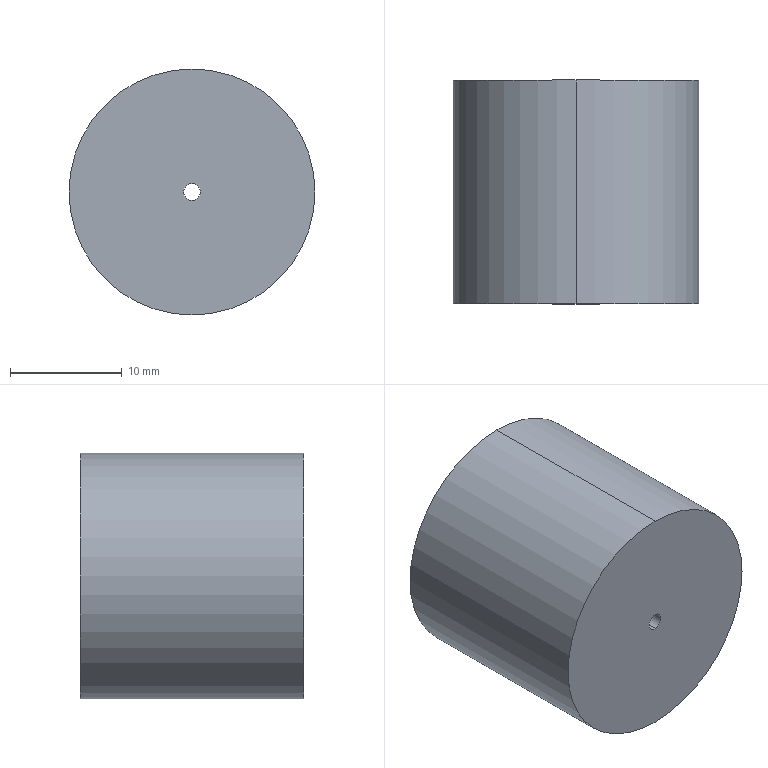Part | 1 solid | 6 faces | box 22 x 20 x 22 mm | volume 7567 mm3 | cylinder 4 | plane 2 | commonest cylinder face diameters 1.5 x2 22 x2
STEP:
#1=CARTESIAN_POINT('',(0.,20.,-0.75));
#2=VERTEX_POINT('',#1);
#3=CARTESIAN_POINT('',(0.,20.,0.75));
#4=VERTEX_POINT('',#3);
#5=CARTESIAN_POINT('',(0.,20.,0.));
#6=DIRECTION('',(0.,1.,0.));
#7=DIRECTION('',(0.,0.,1.));
#8=AXIS2_PLACEMENT_3D('',#5,#6,#7);
#9=CIRCLE('',#8,0.75);
#10=EDGE_CURVE('',#2,#4,#9,.T.);
#11=ORIENTED_EDGE('',*,*,#10,.T.);
#12=CARTESIAN_POINT('',(0.,0.,0.75));
#13=VERTEX_POINT('',#12);
#14=CARTESIAN_POINT('',(0.,20.,0.75));
#15=DIRECTION('',(0.,-1.,0.));
#16=VECTOR('',#15,1000.);
#17=LINE('',#14,#16);
#18=EDGE_CURVE('',#4,#13,#17,.T.);
#19=ORIENTED_EDGE('',*,*,#18,.T.);
#20=CARTESIAN_POINT('',(0.,0.,-0.75));
#21=VERTEX_POINT('',#20);
#22=CARTESIAN_POINT('',(0.,0.,0.));
#23=DIRECTION('',(0.,1.,0.));
#24=DIRECTION('',(0.,0.,1.));
#25=AXIS2_PLACEMENT_3D('',#22,#23,#24);
#26=CIRCLE('',#25,0.75);
#27=EDGE_CURVE('',#21,#13,#26,.T.);
#28=ORIENTED_EDGE('',*,*,#27,.F.);
#29=CARTESIAN_POINT('',(0.,20.,-0.75));
#30=DIRECTION('',(0.,-1.,0.));
#31=VECTOR('',#30,1000.);
#32=LINE('',#29,#31);
#33=EDGE_CURVE('',#2,#21,#32,.T.);
#34=ORIENTED_EDGE('',*,*,#33,.F.);
#35=EDGE_LOOP('',(#11,#19,#28,#34));
#36=FACE_OUTER_BOUND('',#35,.T.);
#37=CARTESIAN_POINT('',(0.,20.,0.));
#38=DIRECTION('',(0.,-1.,0.));
#39=DIRECTION('',(0.,0.,-1.));
#40=AXIS2_PLACEMENT_3D('',#37,#38,#39);
#41=CYLINDRICAL_SURFACE('',#40,0.75);
#42=ADVANCED_FACE('',(#36),#41,.F.);
#43=CARTESIAN_POINT('',(0.,20.,11.));
#44=VERTEX_POINT('',#43);
#45=CARTESIAN_POINT('',(0.,20.,-11.));
#46=VERTEX_POINT('',#45);
#47=CARTESIAN_POINT('',(0.,20.,0.));
#48=DIRECTION('',(0.,1.,0.));
#49=DIRECTION('',(0.,0.,1.));
#50=AXIS2_PLACEMENT_3D('',#47,#48,#49);
#51=CIRCLE('',#50,11.);
#52=EDGE_CURVE('',#44,#46,#51,.T.);
#53=ORIENTED_EDGE('',*,*,#52,.F.);
#54=CARTESIAN_POINT('',(0.,0.,11.));
#55=VERTEX_POINT('',#54);
#56=CARTESIAN_POINT('',(0.,20.,11.));
#57=DIRECTION('',(0.,-1.,0.));
#58=VECTOR('',#57,1000.);
#59=LINE('',#56,#58);
#60=EDGE_CURVE('',#44,#55,#59,.T.);
#61=ORIENTED_EDGE('',*,*,#60,.T.);
#62=CARTESIAN_POINT('',(0.,0.,-11.));
#63=VERTEX_POINT('',#62);
#64=CARTESIAN_POINT('',(0.,0.,0.));
#65=DIRECTION('',(0.,1.,0.));
#66=DIRECTION('',(0.,0.,1.));
#67=AXIS2_PLACEMENT_3D('',#64,#65,#66);
#68=CIRCLE('',#67,11.);
#69=EDGE_CURVE('',#55,#63,#68,.T.);
#70=ORIENTED_EDGE('',*,*,#69,.T.);
#71=CARTESIAN_POINT('',(0.,20.,-11.));
#72=DIRECTION('',(0.,-1.,0.));
#73=VECTOR('',#72,1000.);
#74=LINE('',#71,#73);
#75=EDGE_CURVE('',#46,#63,#74,.T.);
#76=ORIENTED_EDGE('',*,*,#75,.F.);
#77=EDGE_LOOP('',(#53,#61,#70,#76));
#78=FACE_OUTER_BOUND('',#77,.T.);
#79=CARTESIAN_POINT('',(0.,20.,0.));
#80=DIRECTION('',(0.,-1.,0.));
#81=DIRECTION('',(0.,0.,-1.));
#82=AXIS2_PLACEMENT_3D('',#79,#80,#81);
#83=CYLINDRICAL_SURFACE('',#82,11.);
#84=ADVANCED_FACE('',(#78),#83,.T.);
#85=CARTESIAN_POINT('',(0.,20.,0.));
#86=DIRECTION('',(0.,1.,0.));
#87=DIRECTION('',(0.,0.,1.));
#88=AXIS2_PLACEMENT_3D('',#85,#86,#87);
#89=CIRCLE('',#88,11.);
#90=EDGE_CURVE('',#46,#44,#89,.T.);
#91=ORIENTED_EDGE('',*,*,#90,.T.);
#92=ORIENTED_EDGE('',*,*,#52,.T.);
#93=EDGE_LOOP('',(#91,#92));
#94=FACE_OUTER_BOUND('',#93,.T.);
#95=ORIENTED_EDGE('',*,*,#10,.F.);
#96=CARTESIAN_POINT('',(0.,20.,0.));
#97=DIRECTION('',(0.,1.,0.));
#98=DIRECTION('',(0.,0.,1.));
#99=AXIS2_PLACEMENT_3D('',#96,#97,#98);
#100=CIRCLE('',#99,0.75);
#101=EDGE_CURVE('',#4,#2,#100,.T.);
#102=ORIENTED_EDGE('',*,*,#101,.F.);
#103=EDGE_LOOP('',(#95,#102));
#104=FACE_BOUND('',#103,.T.);
#105=CARTESIAN_POINT('',(0.,20.,0.));
#106=DIRECTION('',(0.,1.,0.));
#107=DIRECTION('',(0.,0.,1.));
#108=AXIS2_PLACEMENT_3D('',#105,#106,#107);
#109=PLANE('',#108);
#110=ADVANCED_FACE('',(#94,#104),#109,.T.);
#111=CARTESIAN_POINT('',(0.,0.,0.));
#112=DIRECTION('',(0.,1.,0.));
#113=DIRECTION('',(0.,0.,1.));
#114=AXIS2_PLACEMENT_3D('',#111,#112,#113);
#115=CIRCLE('',#114,11.);
#116=EDGE_CURVE('',#63,#55,#115,.T.);
#117=ORIENTED_EDGE('',*,*,#116,.F.);
#118=ORIENTED_EDGE('',*,*,#69,.F.);
#119=EDGE_LOOP('',(#117,#118));
#120=FACE_OUTER_BOUND('',#119,.T.);
#121=ORIENTED_EDGE('',*,*,#27,.T.);
#122=CARTESIAN_POINT('',(0.,0.,0.));
#123=DIRECTION('',(0.,1.,0.));
#124=DIRECTION('',(0.,0.,1.));
#125=AXIS2_PLACEMENT_3D('',#122,#123,#124);
#126=CIRCLE('',#125,0.75);
#127=EDGE_CURVE('',#13,#21,#126,.T.);
#128=ORIENTED_EDGE('',*,*,#127,.T.);
#129=EDGE_LOOP('',(#121,#128));
#130=FACE_BOUND('',#129,.T.);
#131=CARTESIAN_POINT('',(0.,0.,0.));
#132=DIRECTION('',(0.,1.,0.));
#133=DIRECTION('',(0.,0.,1.));
#134=AXIS2_PLACEMENT_3D('',#131,#132,#133);
#135=PLANE('',#134);
#136=ADVANCED_FACE('',(#120,#130),#135,.F.);
#137=ORIENTED_EDGE('',*,*,#60,.F.);
#138=ORIENTED_EDGE('',*,*,#90,.F.);
#139=ORIENTED_EDGE('',*,*,#75,.T.);
#140=ORIENTED_EDGE('',*,*,#116,.T.);
#141=EDGE_LOOP('',(#137,#138,#139,#140));
#142=FACE_OUTER_BOUND('',#141,.T.);
#143=CARTESIAN_POINT('',(0.,20.,0.));
#144=DIRECTION('',(0.,-1.,0.));
#145=DIRECTION('',(0.,0.,-1.));
#146=AXIS2_PLACEMENT_3D('',#143,#144,#145);
#147=CYLINDRICAL_SURFACE('',#146,11.);
#148=ADVANCED_FACE('',(#142),#147,.T.);
#149=ORIENTED_EDGE('',*,*,#18,.F.);
#150=ORIENTED_EDGE('',*,*,#101,.T.);
#151=ORIENTED_EDGE('',*,*,#33,.T.);
#152=ORIENTED_EDGE('',*,*,#127,.F.);
#153=EDGE_LOOP('',(#149,#150,#151,#152));
#154=FACE_OUTER_BOUND('',#153,.T.);
#155=CARTESIAN_POINT('',(0.,20.,0.));
#156=DIRECTION('',(0.,-1.,0.));
#157=DIRECTION('',(0.,0.,-1.));
#158=AXIS2_PLACEMENT_3D('',#155,#156,#157);
#159=CYLINDRICAL_SURFACE('',#158,0.75);
#160=ADVANCED_FACE('',(#154),#159,.F.);
#161=CLOSED_SHELL('',(#42,#84,#110,#136,#148,#160));
#162=MANIFOLD_SOLID_BREP('',#161);
#163=CARTESIAN_POINT('',(0.,0.,0.));
#164=DIRECTION('',(0.,0.,1.));
#165=DIRECTION('',(1.,0.,0.));
#166=AXIS2_PLACEMENT_3D('',#163,#164,#165);
#167=(LENGTH_UNIT()NAMED_UNIT(*)SI_UNIT(.MILLI.,.METRE.));
#168=UNCERTAINTY_MEASURE_WITH_UNIT(LENGTH_MEASURE(0.00001),#167,'','');
#169=(NAMED_UNIT(*)PLANE_ANGLE_UNIT()SI_UNIT($,.RADIAN.));
#170=(NAMED_UNIT(*)SI_UNIT($,.STERADIAN.)SOLID_ANGLE_UNIT());
#171=(GEOMETRIC_REPRESENTATION_CONTEXT(3)GLOBAL_UNCERTAINTY_ASSIGNED_CONTEXT((#168))GLOBAL_UNIT_ASSIGNED_CONTEXT((#167,#169,#170))REPRESENTATION_CONTEXT('',''));
#172=ADVANCED_BREP_SHAPE_REPRESENTATION('',(#162,#166),#171);